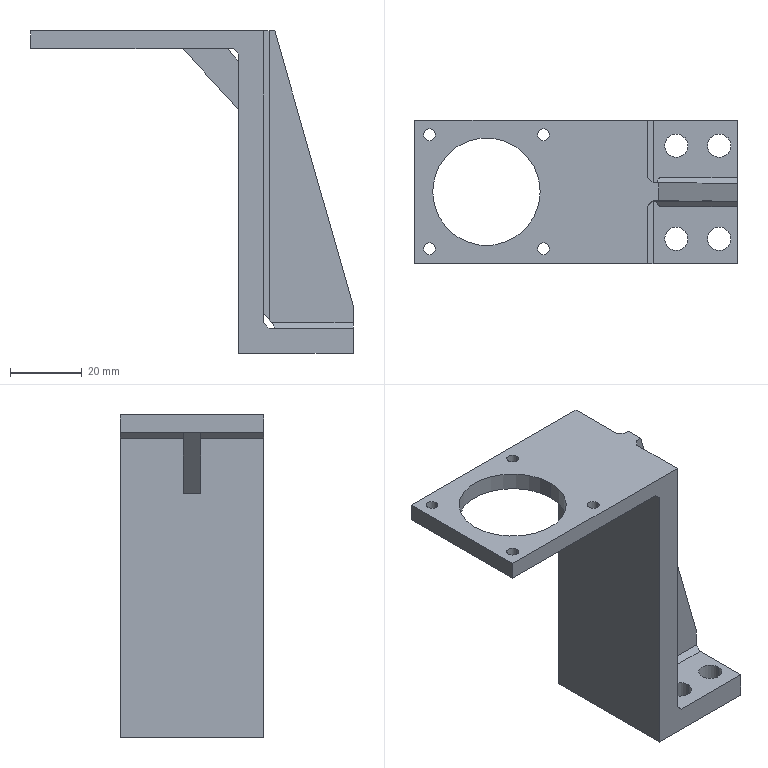Part | Creo | features CURVE 6, PROTRUSION 4, DATUM PLANE 3, CUT 2, CHAMFER 1, COORDINATE SYSTEM 1 | 1 solid | 42 faces | box 90 x 40 x 90 mm | volume 46256 mm3 | plane 24 | cylinder 18 | commonest cylinder face diameters 3.3 x8 6.5 x8 30 x2
STEP:
#1=CARTESIAN_POINT('',(0.,0.,0.));
#2=DIRECTION('',(0.,0.,1.));
#3=DIRECTION('',(1.,0.,0.));
#4=AXIS2_PLACEMENT_3D('',#1,#2,#3);
#5=CARTESIAN_POINT('',(36.5,-20.,0.));
#6=VERTEX_POINT('',#5);
#7=CARTESIAN_POINT('',(36.5,20.,0.));
#8=VERTEX_POINT('',#7);
#9=CARTESIAN_POINT('',(36.5,-20.,0.));
#10=DIRECTION('',(0.,1.,0.));
#11=VECTOR('',#10,40.);
#12=LINE('',#9,#11);
#13=EDGE_CURVE('',#6,#8,#12,.T.);
#14=ORIENTED_EDGE('',*,*,#13,.T.);
#15=CARTESIAN_POINT('',(-20.,20.,0.));
#16=VERTEX_POINT('',#15);
#17=CARTESIAN_POINT('',(36.5,20.,0.));
#18=DIRECTION('',(-1.,0.,0.));
#19=VECTOR('',#18,56.5);
#20=LINE('',#17,#19);
#21=EDGE_CURVE('',#8,#16,#20,.T.);
#22=ORIENTED_EDGE('',*,*,#21,.T.);
#23=CARTESIAN_POINT('',(-20.,-20.,0.));
#24=VERTEX_POINT('',#23);
#25=CARTESIAN_POINT('',(-20.,20.,0.));
#26=DIRECTION('',(0.,-1.,0.));
#27=VECTOR('',#26,40.);
#28=LINE('',#25,#27);
#29=EDGE_CURVE('',#16,#24,#28,.T.);
#30=ORIENTED_EDGE('',*,*,#29,.T.);
#31=CARTESIAN_POINT('',(-20.,-20.,0.));
#32=DIRECTION('',(1.,0.,0.));
#33=VECTOR('',#32,56.5);
#34=LINE('',#31,#33);
#35=EDGE_CURVE('',#24,#6,#34,.T.);
#36=ORIENTED_EDGE('',*,*,#35,.T.);
#37=EDGE_LOOP('',(#14,#22,#30,#36));
#38=FACE_OUTER_BOUND('',#37,.F.);
#39=CARTESIAN_POINT('',(17.56,15.91,0.));
#40=VERTEX_POINT('',#39);
#41=CARTESIAN_POINT('',(14.26,15.91,0.));
#42=VERTEX_POINT('',#41);
#43=CARTESIAN_POINT('',(15.91,15.91,0.));
#44=DIRECTION('',(0.,0.,-1.));
#45=DIRECTION('',(1.,0.,0.));
#46=AXIS2_PLACEMENT_3D('',#43,#44,#45);
#47=CIRCLE('',#46,1.65);
#48=EDGE_CURVE('',#40,#42,#47,.T.);
#49=ORIENTED_EDGE('',*,*,#48,.T.);
#50=CARTESIAN_POINT('',(15.91,15.91,0.));
#51=DIRECTION('',(0.,0.,-1.));
#52=DIRECTION('',(-1.,0.,0.));
#53=AXIS2_PLACEMENT_3D('',#50,#51,#52);
#54=CIRCLE('',#53,1.65);
#55=EDGE_CURVE('',#42,#40,#54,.T.);
#56=ORIENTED_EDGE('',*,*,#55,.T.);
#57=EDGE_LOOP('',(#49,#56));
#58=FACE_BOUND('',#57,.F.);
#59=CARTESIAN_POINT('',(-14.26,15.91,0.));
#60=VERTEX_POINT('',#59);
#61=CARTESIAN_POINT('',(-17.56,15.91,0.));
#62=VERTEX_POINT('',#61);
#63=CARTESIAN_POINT('',(-15.91,15.91,0.));
#64=DIRECTION('',(0.,0.,-1.));
#65=DIRECTION('',(1.,0.,0.));
#66=AXIS2_PLACEMENT_3D('',#63,#64,#65);
#67=CIRCLE('',#66,1.65);
#68=EDGE_CURVE('',#60,#62,#67,.T.);
#69=ORIENTED_EDGE('',*,*,#68,.T.);
#70=CARTESIAN_POINT('',(-15.91,15.91,0.));
#71=DIRECTION('',(0.,0.,-1.));
#72=DIRECTION('',(-1.,0.,0.));
#73=AXIS2_PLACEMENT_3D('',#70,#71,#72);
#74=CIRCLE('',#73,1.65);
#75=EDGE_CURVE('',#62,#60,#74,.T.);
#76=ORIENTED_EDGE('',*,*,#75,.T.);
#77=EDGE_LOOP('',(#69,#76));
#78=FACE_BOUND('',#77,.F.);
#79=CARTESIAN_POINT('',(-14.26,-15.91,0.));
#80=VERTEX_POINT('',#79);
#81=CARTESIAN_POINT('',(-17.56,-15.91,0.));
#82=VERTEX_POINT('',#81);
#83=CARTESIAN_POINT('',(-15.91,-15.91,0.));
#84=DIRECTION('',(0.,0.,-1.));
#85=DIRECTION('',(1.,0.,0.));
#86=AXIS2_PLACEMENT_3D('',#83,#84,#85);
#87=CIRCLE('',#86,1.65);
#88=EDGE_CURVE('',#80,#82,#87,.T.);
#89=ORIENTED_EDGE('',*,*,#88,.T.);
#90=CARTESIAN_POINT('',(-15.91,-15.91,0.));
#91=DIRECTION('',(0.,0.,-1.));
#92=DIRECTION('',(-1.,0.,0.));
#93=AXIS2_PLACEMENT_3D('',#90,#91,#92);
#94=CIRCLE('',#93,1.65);
#95=EDGE_CURVE('',#82,#80,#94,.T.);
#96=ORIENTED_EDGE('',*,*,#95,.T.);
#97=EDGE_LOOP('',(#89,#96));
#98=FACE_BOUND('',#97,.F.);
#99=CARTESIAN_POINT('',(17.56,-15.91,0.));
#100=VERTEX_POINT('',#99);
#101=CARTESIAN_POINT('',(14.26,-15.91,0.));
#102=VERTEX_POINT('',#101);
#103=CARTESIAN_POINT('',(15.91,-15.91,0.));
#104=DIRECTION('',(0.,0.,-1.));
#105=DIRECTION('',(1.,0.,0.));
#106=AXIS2_PLACEMENT_3D('',#103,#104,#105);
#107=CIRCLE('',#106,1.65);
#108=EDGE_CURVE('',#100,#102,#107,.T.);
#109=ORIENTED_EDGE('',*,*,#108,.T.);
#110=CARTESIAN_POINT('',(15.91,-15.91,0.));
#111=DIRECTION('',(0.,0.,-1.));
#112=DIRECTION('',(-1.,0.,0.));
#113=AXIS2_PLACEMENT_3D('',#110,#111,#112);
#114=CIRCLE('',#113,1.65);
#115=EDGE_CURVE('',#102,#100,#114,.T.);
#116=ORIENTED_EDGE('',*,*,#115,.T.);
#117=EDGE_LOOP('',(#109,#116));
#118=FACE_BOUND('',#117,.F.);
#119=CARTESIAN_POINT('',(34.828,-2.5,0.));
#120=VERTEX_POINT('',#119);
#121=CARTESIAN_POINT('',(22.404,-2.5,0.));
#122=VERTEX_POINT('',#121);
#123=CARTESIAN_POINT('',(34.828,-2.5,0.));
#124=DIRECTION('',(-1.,0.,0.));
#125=VECTOR('',#124,12.424);
#126=LINE('',#123,#125);
#127=EDGE_CURVE('',#120,#122,#126,.T.);
#128=ORIENTED_EDGE('',*,*,#127,.T.);
#129=CARTESIAN_POINT('',(22.404,2.5,0.));
#130=VERTEX_POINT('',#129);
#131=CARTESIAN_POINT('',(22.404,-2.5,0.));
#132=DIRECTION('',(0.,1.,0.));
#133=VECTOR('',#132,5.);
#134=LINE('',#131,#133);
#135=EDGE_CURVE('',#122,#130,#134,.T.);
#136=ORIENTED_EDGE('',*,*,#135,.T.);
#137=CARTESIAN_POINT('',(34.828,2.5,0.));
#138=VERTEX_POINT('',#137);
#139=CARTESIAN_POINT('',(34.828,2.5,0.));
#140=DIRECTION('',(-1.,0.,0.));
#141=VECTOR('',#140,12.424);
#142=LINE('',#139,#141);
#143=EDGE_CURVE('',#138,#130,#142,.T.);
#144=ORIENTED_EDGE('',*,*,#143,.F.);
#145=CARTESIAN_POINT('',(34.828,-2.5,0.));
#146=DIRECTION('',(0.,1.,0.));
#147=VECTOR('',#146,5.);
#148=LINE('',#145,#147);
#149=EDGE_CURVE('',#120,#138,#148,.T.);
#150=ORIENTED_EDGE('',*,*,#149,.F.);
#151=EDGE_LOOP('',(#128,#136,#144,#150));
#152=FACE_BOUND('',#151,.F.);
#153=CARTESIAN_POINT('',(15.,0.,0.));
#154=VERTEX_POINT('',#153);
#155=CARTESIAN_POINT('',(-15.,0.,0.));
#156=VERTEX_POINT('',#155);
#157=CARTESIAN_POINT('',(0.,0.,0.));
#158=DIRECTION('',(0.,0.,-1.));
#159=DIRECTION('',(1.,0.,0.));
#160=AXIS2_PLACEMENT_3D('',#157,#158,#159);
#161=CIRCLE('',#160,15.);
#162=EDGE_CURVE('',#154,#156,#161,.T.);
#163=ORIENTED_EDGE('',*,*,#162,.T.);
#164=CARTESIAN_POINT('',(0.,0.,0.));
#165=DIRECTION('',(0.,0.,-1.));
#166=DIRECTION('',(-1.,0.,0.));
#167=AXIS2_PLACEMENT_3D('',#164,#165,#166);
#168=CIRCLE('',#167,15.);
#169=EDGE_CURVE('',#156,#154,#168,.T.);
#170=ORIENTED_EDGE('',*,*,#169,.T.);
#171=EDGE_LOOP('',(#163,#170));
#172=FACE_BOUND('',#171,.F.);
#173=CARTESIAN_POINT('',(0.,0.,0.));
#174=DIRECTION('',(0.,0.,1.));
#175=DIRECTION('',(1.,0.,0.));
#176=AXIS2_PLACEMENT_3D('',#173,#174,#175);
#177=PLANE('',#176);
#178=ADVANCED_FACE('',(#38,#58,#78,#98,#118,#152,#172),#177,.F.);
#179=ORIENTED_EDGE('',*,*,#162,.F.);
#180=CARTESIAN_POINT('',(15.,0.,5.));
#181=VERTEX_POINT('',#180);
#182=CARTESIAN_POINT('',(15.,0.,0.));
#183=DIRECTION('',(0.,0.,1.));
#184=VECTOR('',#183,5.);
#185=LINE('',#182,#184);
#186=EDGE_CURVE('',#154,#181,#185,.T.);
#187=ORIENTED_EDGE('',*,*,#186,.T.);
#188=CARTESIAN_POINT('',(-15.,0.,5.));
#189=VERTEX_POINT('',#188);
#190=CARTESIAN_POINT('',(0.,0.,5.));
#191=DIRECTION('',(0.,0.,-1.));
#192=DIRECTION('',(1.,0.,0.));
#193=AXIS2_PLACEMENT_3D('',#190,#191,#192);
#194=CIRCLE('',#193,15.);
#195=EDGE_CURVE('',#181,#189,#194,.T.);
#196=ORIENTED_EDGE('',*,*,#195,.T.);
#197=CARTESIAN_POINT('',(-15.,0.,0.));
#198=DIRECTION('',(0.,0.,1.));
#199=VECTOR('',#198,5.);
#200=LINE('',#197,#199);
#201=EDGE_CURVE('',#156,#189,#200,.T.);
#202=ORIENTED_EDGE('',*,*,#201,.F.);
#203=EDGE_LOOP('',(#179,#187,#196,#202));
#204=FACE_OUTER_BOUND('',#203,.F.);
#205=CARTESIAN_POINT('',(0.,0.,0.));
#206=DIRECTION('',(0.,0.,1.));
#207=DIRECTION('',(1.,0.,0.));
#208=AXIS2_PLACEMENT_3D('',#205,#206,#207);
#209=CYLINDRICAL_SURFACE('',#208,15.);
#210=ADVANCED_FACE('',(#204),#209,.F.);
#211=ORIENTED_EDGE('',*,*,#169,.F.);
#212=ORIENTED_EDGE('',*,*,#201,.T.);
#213=CARTESIAN_POINT('',(0.,0.,5.));
#214=DIRECTION('',(0.,0.,-1.));
#215=DIRECTION('',(-1.,0.,0.));
#216=AXIS2_PLACEMENT_3D('',#213,#214,#215);
#217=CIRCLE('',#216,15.);
#218=EDGE_CURVE('',#189,#181,#217,.T.);
#219=ORIENTED_EDGE('',*,*,#218,.T.);
#220=ORIENTED_EDGE('',*,*,#186,.F.);
#221=EDGE_LOOP('',(#211,#212,#219,#220));
#222=FACE_OUTER_BOUND('',#221,.F.);
#223=CARTESIAN_POINT('',(0.,0.,0.));
#224=DIRECTION('',(0.,0.,1.));
#225=DIRECTION('',(1.,0.,0.));
#226=AXIS2_PLACEMENT_3D('',#223,#224,#225);
#227=CYLINDRICAL_SURFACE('',#226,15.);
#228=ADVANCED_FACE('',(#222),#227,.F.);
#229=CARTESIAN_POINT('',(45.,20.,5.));
#230=VERTEX_POINT('',#229);
#231=CARTESIAN_POINT('',(45.,4.,5.));
#232=VERTEX_POINT('',#231);
#233=CARTESIAN_POINT('',(45.,20.,5.));
#234=DIRECTION('',(0.,-1.,0.));
#235=VECTOR('',#234,16.);
#236=LINE('',#233,#235);
#237=EDGE_CURVE('',#230,#232,#236,.T.);
#238=ORIENTED_EDGE('',*,*,#237,.T.);
#239=CARTESIAN_POINT('',(46.5,2.5,5.));
#240=VERTEX_POINT('',#239);
#241=CARTESIAN_POINT('',(46.5,2.5,5.));
#242=DIRECTION('',(-0.7071,0.7071,0.));
#243=VECTOR('',#242,2.121);
#244=LINE('',#241,#243);
#245=EDGE_CURVE('',#240,#232,#244,.T.);
#246=ORIENTED_EDGE('',*,*,#245,.F.);
#247=CARTESIAN_POINT('',(48.097,2.5,5.));
#248=VERTEX_POINT('',#247);
#249=CARTESIAN_POINT('',(46.5,2.5,5.));
#250=DIRECTION('',(1.,0.,0.));
#251=VECTOR('',#250,1.597);
#252=LINE('',#249,#251);
#253=EDGE_CURVE('',#240,#248,#252,.T.);
#254=ORIENTED_EDGE('',*,*,#253,.T.);
#255=CARTESIAN_POINT('',(48.097,-2.5,5.));
#256=VERTEX_POINT('',#255);
#257=CARTESIAN_POINT('',(48.097,-2.5,5.));
#258=DIRECTION('',(0.,1.,0.));
#259=VECTOR('',#258,5.);
#260=LINE('',#257,#259);
#261=EDGE_CURVE('',#256,#248,#260,.T.);
#262=ORIENTED_EDGE('',*,*,#261,.F.);
#263=CARTESIAN_POINT('',(46.5,-2.5,5.));
#264=VERTEX_POINT('',#263);
#265=CARTESIAN_POINT('',(46.5,-2.5,5.));
#266=DIRECTION('',(1.,0.,0.));
#267=VECTOR('',#266,1.597);
#268=LINE('',#265,#267);
#269=EDGE_CURVE('',#264,#256,#268,.T.);
#270=ORIENTED_EDGE('',*,*,#269,.F.);
#271=CARTESIAN_POINT('',(45.,-4.,5.));
#272=VERTEX_POINT('',#271);
#273=CARTESIAN_POINT('',(45.,-4.,5.));
#274=DIRECTION('',(0.7071,0.7071,0.));
#275=VECTOR('',#274,2.121);
#276=LINE('',#273,#275);
#277=EDGE_CURVE('',#272,#264,#276,.T.);
#278=ORIENTED_EDGE('',*,*,#277,.F.);
#279=CARTESIAN_POINT('',(45.,-20.,5.));
#280=VERTEX_POINT('',#279);
#281=CARTESIAN_POINT('',(45.,-4.,5.));
#282=DIRECTION('',(0.,-1.,0.));
#283=VECTOR('',#282,16.);
#284=LINE('',#281,#283);
#285=EDGE_CURVE('',#272,#280,#284,.T.);
#286=ORIENTED_EDGE('',*,*,#285,.T.);
#287=CARTESIAN_POINT('',(-20.,-20.,5.));
#288=VERTEX_POINT('',#287);
#289=CARTESIAN_POINT('',(45.,-20.,5.));
#290=DIRECTION('',(-1.,0.,0.));
#291=VECTOR('',#290,65.);
#292=LINE('',#289,#291);
#293=EDGE_CURVE('',#280,#288,#292,.T.);
#294=ORIENTED_EDGE('',*,*,#293,.T.);
#295=CARTESIAN_POINT('',(-20.,20.,5.));
#296=VERTEX_POINT('',#295);
#297=CARTESIAN_POINT('',(-20.,20.,5.));
#298=DIRECTION('',(0.,-1.,0.));
#299=VECTOR('',#298,40.);
#300=LINE('',#297,#299);
#301=EDGE_CURVE('',#296,#288,#300,.T.);
#302=ORIENTED_EDGE('',*,*,#301,.F.);
#303=CARTESIAN_POINT('',(-20.,20.,5.));
#304=DIRECTION('',(1.,0.,0.));
#305=VECTOR('',#304,65.);
#306=LINE('',#303,#305);
#307=EDGE_CURVE('',#296,#230,#306,.T.);
#308=ORIENTED_EDGE('',*,*,#307,.T.);
#309=EDGE_LOOP('',(#238,#246,#254,#262,#270,#278,#286,#294,#302,#308));
#310=FACE_OUTER_BOUND('',#309,.F.);
#311=CARTESIAN_POINT('',(17.56,15.91,5.));
#312=VERTEX_POINT('',#311);
#313=CARTESIAN_POINT('',(14.26,15.91,5.));
#314=VERTEX_POINT('',#313);
#315=CARTESIAN_POINT('',(15.91,15.91,5.));
#316=DIRECTION('',(0.,0.,-1.));
#317=DIRECTION('',(1.,0.,0.));
#318=AXIS2_PLACEMENT_3D('',#315,#316,#317);
#319=CIRCLE('',#318,1.65);
#320=EDGE_CURVE('',#312,#314,#319,.T.);
#321=ORIENTED_EDGE('',*,*,#320,.F.);
#322=CARTESIAN_POINT('',(15.91,15.91,5.));
#323=DIRECTION('',(0.,0.,-1.));
#324=DIRECTION('',(-1.,0.,0.));
#325=AXIS2_PLACEMENT_3D('',#322,#323,#324);
#326=CIRCLE('',#325,1.65);
#327=EDGE_CURVE('',#314,#312,#326,.T.);
#328=ORIENTED_EDGE('',*,*,#327,.F.);
#329=EDGE_LOOP('',(#321,#328));
#330=FACE_BOUND('',#329,.F.);
#331=CARTESIAN_POINT('',(-14.26,15.91,5.));
#332=VERTEX_POINT('',#331);
#333=CARTESIAN_POINT('',(-17.56,15.91,5.));
#334=VERTEX_POINT('',#333);
#335=CARTESIAN_POINT('',(-15.91,15.91,5.));
#336=DIRECTION('',(0.,0.,-1.));
#337=DIRECTION('',(1.,0.,0.));
#338=AXIS2_PLACEMENT_3D('',#335,#336,#337);
#339=CIRCLE('',#338,1.65);
#340=EDGE_CURVE('',#332,#334,#339,.T.);
#341=ORIENTED_EDGE('',*,*,#340,.F.);
#342=CARTESIAN_POINT('',(-15.91,15.91,5.));
#343=DIRECTION('',(0.,0.,-1.));
#344=DIRECTION('',(-1.,0.,0.));
#345=AXIS2_PLACEMENT_3D('',#342,#343,#344);
#346=CIRCLE('',#345,1.65);
#347=EDGE_CURVE('',#334,#332,#346,.T.);
#348=ORIENTED_EDGE('',*,*,#347,.F.);
#349=EDGE_LOOP('',(#341,#348));
#350=FACE_BOUND('',#349,.F.);
#351=CARTESIAN_POINT('',(-14.26,-15.91,5.));
#352=VERTEX_POINT('',#351);
#353=CARTESIAN_POINT('',(-17.56,-15.91,5.));
#354=VERTEX_POINT('',#353);
#355=CARTESIAN_POINT('',(-15.91,-15.91,5.));
#356=DIRECTION('',(0.,0.,-1.));
#357=DIRECTION('',(1.,0.,0.));
#358=AXIS2_PLACEMENT_3D('',#355,#356,#357);
#359=CIRCLE('',#358,1.65);
#360=EDGE_CURVE('',#352,#354,#359,.T.);
#361=ORIENTED_EDGE('',*,*,#360,.F.);
#362=CARTESIAN_POINT('',(-15.91,-15.91,5.));
#363=DIRECTION('',(0.,0.,-1.));
#364=DIRECTION('',(-1.,0.,0.));
#365=AXIS2_PLACEMENT_3D('',#362,#363,#364);
#366=CIRCLE('',#365,1.65);
#367=EDGE_CURVE('',#354,#352,#366,.T.);
#368=ORIENTED_EDGE('',*,*,#367,.F.);
#369=EDGE_LOOP('',(#361,#368));
#370=FACE_BOUND('',#369,.F.);
#371=CARTESIAN_POINT('',(17.56,-15.91,5.));
#372=VERTEX_POINT('',#371);
#373=CARTESIAN_POINT('',(14.26,-15.91,5.));
#374=VERTEX_POINT('',#373);
#375=CARTESIAN_POINT('',(15.91,-15.91,5.));
#376=DIRECTION('',(0.,0.,-1.));
#377=DIRECTION('',(1.,0.,0.));
#378=AXIS2_PLACEMENT_3D('',#375,#376,#377);
#379=CIRCLE('',#378,1.65);
#380=EDGE_CURVE('',#372,#374,#379,.T.);
#381=ORIENTED_EDGE('',*,*,#380,.F.);
#382=CARTESIAN_POINT('',(15.91,-15.91,5.));
#383=DIRECTION('',(0.,0.,-1.));
#384=DIRECTION('',(-1.,0.,0.));
#385=AXIS2_PLACEMENT_3D('',#382,#383,#384);
#386=CIRCLE('',#385,1.65);
#387=EDGE_CURVE('',#374,#372,#386,.T.);
#388=ORIENTED_EDGE('',*,*,#387,.F.);
#389=EDGE_LOOP('',(#381,#388));
#390=FACE_BOUND('',#389,.F.);
#391=ORIENTED_EDGE('',*,*,#195,.F.);
#392=ORIENTED_EDGE('',*,*,#218,.F.);
#393=EDGE_LOOP('',(#391,#392));
#394=FACE_BOUND('',#393,.F.);
#395=CARTESIAN_POINT('',(0.,0.,5.));
#396=DIRECTION('',(0.,0.,1.));
#397=DIRECTION('',(1.,0.,0.));
#398=AXIS2_PLACEMENT_3D('',#395,#396,#397);
#399=PLANE('',#398);
#400=ADVANCED_FACE('',(#310,#330,#350,#370,#390,#394),#399,.T.);
#401=ORIENTED_EDGE('',*,*,#48,.F.);
#402=CARTESIAN_POINT('',(17.56,15.91,0.));
#403=DIRECTION('',(0.,0.,1.));
#404=VECTOR('',#403,5.);
#405=LINE('',#402,#404);
#406=EDGE_CURVE('',#40,#312,#405,.T.);
#407=ORIENTED_EDGE('',*,*,#406,.T.);
#408=ORIENTED_EDGE('',*,*,#320,.T.);
#409=CARTESIAN_POINT('',(14.26,15.91,0.));
#410=DIRECTION('',(0.,0.,1.));
#411=VECTOR('',#410,5.);
#412=LINE('',#409,#411);
#413=EDGE_CURVE('',#42,#314,#412,.T.);
#414=ORIENTED_EDGE('',*,*,#413,.F.);
#415=EDGE_LOOP('',(#401,#407,#408,#414));
#416=FACE_OUTER_BOUND('',#415,.F.);
#417=CARTESIAN_POINT('',(15.91,15.91,0.));
#418=DIRECTION('',(0.,0.,1.));
#419=DIRECTION('',(1.,0.,0.));
#420=AXIS2_PLACEMENT_3D('',#417,#418,#419);
#421=CYLINDRICAL_SURFACE('',#420,1.65);
#422=ADVANCED_FACE('',(#416),#421,.F.);
#423=ORIENTED_EDGE('',*,*,#55,.F.);
#424=ORIENTED_EDGE('',*,*,#413,.T.);
#425=ORIENTED_EDGE('',*,*,#327,.T.);
#426=ORIENTED_EDGE('',*,*,#406,.F.);
#427=EDGE_LOOP('',(#423,#424,#425,#426));
#428=FACE_OUTER_BOUND('',#427,.F.);
#429=CARTESIAN_POINT('',(15.91,15.91,0.));
#430=DIRECTION('',(0.,0.,1.));
#431=DIRECTION('',(1.,0.,0.));
#432=AXIS2_PLACEMENT_3D('',#429,#430,#431);
#433=CYLINDRICAL_SURFACE('',#432,1.65);
#434=ADVANCED_FACE('',(#428),#433,.F.);
#435=ORIENTED_EDGE('',*,*,#68,.F.);
#436=CARTESIAN_POINT('',(-14.26,15.91,0.));
#437=DIRECTION('',(0.,0.,1.));
#438=VECTOR('',#437,5.);
#439=LINE('',#436,#438);
#440=EDGE_CURVE('',#60,#332,#439,.T.);
#441=ORIENTED_EDGE('',*,*,#440,.T.);
#442=ORIENTED_EDGE('',*,*,#340,.T.);
#443=CARTESIAN_POINT('',(-17.56,15.91,0.));
#444=DIRECTION('',(0.,0.,1.));
#445=VECTOR('',#444,5.);
#446=LINE('',#443,#445);
#447=EDGE_CURVE('',#62,#334,#446,.T.);
#448=ORIENTED_EDGE('',*,*,#447,.F.);
#449=EDGE_LOOP('',(#435,#441,#442,#448));
#450=FACE_OUTER_BOUND('',#449,.F.);
#451=CARTESIAN_POINT('',(-15.91,15.91,0.));
#452=DIRECTION('',(0.,0.,1.));
#453=DIRECTION('',(1.,0.,0.));
#454=AXIS2_PLACEMENT_3D('',#451,#452,#453);
#455=CYLINDRICAL_SURFACE('',#454,1.65);
#456=ADVANCED_FACE('',(#450),#455,.F.);
#457=ORIENTED_EDGE('',*,*,#75,.F.);
#458=ORIENTED_EDGE('',*,*,#447,.T.);
#459=ORIENTED_EDGE('',*,*,#347,.T.);
#460=ORIENTED_EDGE('',*,*,#440,.F.);
#461=EDGE_LOOP('',(#457,#458,#459,#460));
#462=FACE_OUTER_BOUND('',#461,.F.);
#463=CARTESIAN_POINT('',(-15.91,15.91,0.));
#464=DIRECTION('',(0.,0.,1.));
#465=DIRECTION('',(1.,0.,0.));
#466=AXIS2_PLACEMENT_3D('',#463,#464,#465);
#467=CYLINDRICAL_SURFACE('',#466,1.65);
#468=ADVANCED_FACE('',(#462),#467,.F.);
#469=ORIENTED_EDGE('',*,*,#88,.F.);
#470=CARTESIAN_POINT('',(-14.26,-15.91,0.));
#471=DIRECTION('',(0.,0.,1.));
#472=VECTOR('',#471,5.);
#473=LINE('',#470,#472);
#474=EDGE_CURVE('',#80,#352,#473,.T.);
#475=ORIENTED_EDGE('',*,*,#474,.T.);
#476=ORIENTED_EDGE('',*,*,#360,.T.);
#477=CARTESIAN_POINT('',(-17.56,-15.91,0.));
#478=DIRECTION('',(0.,0.,1.));
#479=VECTOR('',#478,5.);
#480=LINE('',#477,#479);
#481=EDGE_CURVE('',#82,#354,#480,.T.);
#482=ORIENTED_EDGE('',*,*,#481,.F.);
#483=EDGE_LOOP('',(#469,#475,#476,#482));
#484=FACE_OUTER_BOUND('',#483,.F.);
#485=CARTESIAN_POINT('',(-15.91,-15.91,0.));
#486=DIRECTION('',(0.,0.,1.));
#487=DIRECTION('',(1.,0.,0.));
#488=AXIS2_PLACEMENT_3D('',#485,#486,#487);
#489=CYLINDRICAL_SURFACE('',#488,1.65);
#490=ADVANCED_FACE('',(#484),#489,.F.);
#491=ORIENTED_EDGE('',*,*,#95,.F.);
#492=ORIENTED_EDGE('',*,*,#481,.T.);
#493=ORIENTED_EDGE('',*,*,#367,.T.);
#494=ORIENTED_EDGE('',*,*,#474,.F.);
#495=EDGE_LOOP('',(#491,#492,#493,#494));
#496=FACE_OUTER_BOUND('',#495,.F.);
#497=CARTESIAN_POINT('',(-15.91,-15.91,0.));
#498=DIRECTION('',(0.,0.,1.));
#499=DIRECTION('',(1.,0.,0.));
#500=AXIS2_PLACEMENT_3D('',#497,#498,#499);
#501=CYLINDRICAL_SURFACE('',#500,1.65);
#502=ADVANCED_FACE('',(#496),#501,.F.);
#503=ORIENTED_EDGE('',*,*,#108,.F.);
#504=CARTESIAN_POINT('',(17.56,-15.91,0.));
#505=DIRECTION('',(0.,0.,1.));
#506=VECTOR('',#505,5.);
#507=LINE('',#504,#506);
#508=EDGE_CURVE('',#100,#372,#507,.T.);
#509=ORIENTED_EDGE('',*,*,#508,.T.);
#510=ORIENTED_EDGE('',*,*,#380,.T.);
#511=CARTESIAN_POINT('',(14.26,-15.91,0.));
#512=DIRECTION('',(0.,0.,1.));
#513=VECTOR('',#512,5.);
#514=LINE('',#511,#513);
#515=EDGE_CURVE('',#102,#374,#514,.T.);
#516=ORIENTED_EDGE('',*,*,#515,.F.);
#517=EDGE_LOOP('',(#503,#509,#510,#516));
#518=FACE_OUTER_BOUND('',#517,.F.);
#519=CARTESIAN_POINT('',(15.91,-15.91,0.));
#520=DIRECTION('',(0.,0.,1.));
#521=DIRECTION('',(1.,0.,0.));
#522=AXIS2_PLACEMENT_3D('',#519,#520,#521);
#523=CYLINDRICAL_SURFACE('',#522,1.65);
#524=ADVANCED_FACE('',(#518),#523,.F.);
#525=ORIENTED_EDGE('',*,*,#115,.F.);
#526=ORIENTED_EDGE('',*,*,#515,.T.);
#527=ORIENTED_EDGE('',*,*,#387,.T.);
#528=ORIENTED_EDGE('',*,*,#508,.F.);
#529=EDGE_LOOP('',(#525,#526,#527,#528));
#530=FACE_OUTER_BOUND('',#529,.F.);
#531=CARTESIAN_POINT('',(15.91,-15.91,0.));
#532=DIRECTION('',(0.,0.,1.));
#533=DIRECTION('',(1.,0.,0.));
#534=AXIS2_PLACEMENT_3D('',#531,#532,#533);
#535=CYLINDRICAL_SURFACE('',#534,1.65);
#536=ADVANCED_FACE('',(#530),#535,.F.);
#537=CARTESIAN_POINT('',(45.,20.,-76.5));
#538=VERTEX_POINT('',#537);
#539=CARTESIAN_POINT('',(45.,-20.,-76.5));
#540=VERTEX_POINT('',#539);
#541=CARTESIAN_POINT('',(45.,20.,-76.5));
#542=DIRECTION('',(0.,-1.,0.));
#543=VECTOR('',#542,40.);
#544=LINE('',#541,#543);
#545=EDGE_CURVE('',#538,#540,#544,.T.);
#546=ORIENTED_EDGE('',*,*,#545,.T.);
#547=CARTESIAN_POINT('',(45.,-20.,5.));
#548=DIRECTION('',(0.,0.,-1.));
#549=VECTOR('',#548,81.5);
#550=LINE('',#547,#549);
#551=EDGE_CURVE('',#280,#540,#550,.T.);
#552=ORIENTED_EDGE('',*,*,#551,.F.);
#553=ORIENTED_EDGE('',*,*,#285,.F.);
#554=CARTESIAN_POINT('',(45.,-4.,-73.824));
#555=VERTEX_POINT('',#554);
#556=CARTESIAN_POINT('',(45.,-4.,5.));
#557=DIRECTION('',(0.,0.,-1.));
#558=VECTOR('',#557,78.824);
#559=LINE('',#556,#558);
#560=EDGE_CURVE('',#272,#555,#559,.T.);
#561=ORIENTED_EDGE('',*,*,#560,.T.);
#562=CARTESIAN_POINT('',(45.,4.,-73.824));
#563=VERTEX_POINT('',#562);
#564=CARTESIAN_POINT('',(45.,4.,-73.824));
#565=DIRECTION('',(0.,-1.,0.));
#566=VECTOR('',#565,8.);
#567=LINE('',#564,#566);
#568=EDGE_CURVE('',#563,#555,#567,.T.);
#569=ORIENTED_EDGE('',*,*,#568,.F.);
#570=CARTESIAN_POINT('',(45.,4.,-73.824));
#571=DIRECTION('',(0.,0.,1.));
#572=VECTOR('',#571,78.824);
#573=LINE('',#570,#572);
#574=EDGE_CURVE('',#563,#232,#573,.T.);
#575=ORIENTED_EDGE('',*,*,#574,.T.);
#576=ORIENTED_EDGE('',*,*,#237,.F.);
#577=CARTESIAN_POINT('',(45.,20.,-76.5));
#578=DIRECTION('',(0.,0.,1.));
#579=VECTOR('',#578,81.5);
#580=LINE('',#577,#579);
#581=EDGE_CURVE('',#538,#230,#580,.T.);
#582=ORIENTED_EDGE('',*,*,#581,.F.);
#583=EDGE_LOOP('',(#546,#552,#553,#561,#569,#575,#576,#582));
#584=FACE_OUTER_BOUND('',#583,.F.);
#585=CARTESIAN_POINT('',(45.,0.,0.));
#586=DIRECTION('',(1.,0.,0.));
#587=DIRECTION('',(0.,1.,0.));
#588=AXIS2_PLACEMENT_3D('',#585,#586,#587);
#589=PLANE('',#588);
#590=ADVANCED_FACE('',(#584),#589,.T.);
#591=ORIENTED_EDGE('',*,*,#545,.F.);
#592=CARTESIAN_POINT('',(46.5,20.,-78.));
#593=VERTEX_POINT('',#592);
#594=CARTESIAN_POINT('',(45.,20.,-76.5));
#595=DIRECTION('',(0.7071,0.,-0.7071));
#596=VECTOR('',#595,2.121);
#597=LINE('',#594,#596);
#598=EDGE_CURVE('',#538,#593,#597,.T.);
#599=ORIENTED_EDGE('',*,*,#598,.T.);
#600=CARTESIAN_POINT('',(46.5,-20.,-78.));
#601=VERTEX_POINT('',#600);
#602=CARTESIAN_POINT('',(46.5,20.,-78.));
#603=DIRECTION('',(0.,-1.,0.));
#604=VECTOR('',#603,40.);
#605=LINE('',#602,#604);
#606=EDGE_CURVE('',#593,#601,#605,.T.);
#607=ORIENTED_EDGE('',*,*,#606,.T.);
#608=CARTESIAN_POINT('',(46.5,-20.,-78.));
#609=DIRECTION('',(-0.7071,0.,0.7071));
#610=VECTOR('',#609,2.121);
#611=LINE('',#608,#610);
#612=EDGE_CURVE('',#601,#540,#611,.T.);
#613=ORIENTED_EDGE('',*,*,#612,.T.);
#614=EDGE_LOOP('',(#591,#599,#607,#613));
#615=FACE_OUTER_BOUND('',#614,.F.);
#616=CARTESIAN_POINT('',(45.75,0.,-77.25));
#617=DIRECTION('',(0.7071,0.,0.7071));
#618=DIRECTION('',(-0.7071,0.,0.7071));
#619=AXIS2_PLACEMENT_3D('',#616,#617,#618);
#620=PLANE('',#619);
#621=ADVANCED_FACE('',(#615),#620,.T.);
#622=ORIENTED_EDGE('',*,*,#21,.F.);
#623=CARTESIAN_POINT('',(38.,20.,-1.5));
#624=VERTEX_POINT('',#623);
#625=CARTESIAN_POINT('',(38.,20.,-1.5));
#626=DIRECTION('',(-0.7071,0.,0.7071));
#627=VECTOR('',#626,2.121);
#628=LINE('',#625,#627);
#629=EDGE_CURVE('',#624,#8,#628,.T.);
#630=ORIENTED_EDGE('',*,*,#629,.F.);
#631=CARTESIAN_POINT('',(38.,20.,-85.));
#632=VERTEX_POINT('',#631);
#633=CARTESIAN_POINT('',(38.,20.,-85.));
#634=DIRECTION('',(0.,0.,1.));
#635=VECTOR('',#634,83.5);
#636=LINE('',#633,#635);
#637=EDGE_CURVE('',#632,#624,#636,.T.);
#638=ORIENTED_EDGE('',*,*,#637,.F.);
#639=CARTESIAN_POINT('',(70.,20.,-85.));
#640=VERTEX_POINT('',#639);
#641=CARTESIAN_POINT('',(38.,20.,-85.));
#642=DIRECTION('',(1.,0.,0.));
#643=VECTOR('',#642,32.);
#644=LINE('',#641,#643);
#645=EDGE_CURVE('',#632,#640,#644,.T.);
#646=ORIENTED_EDGE('',*,*,#645,.T.);
#647=CARTESIAN_POINT('',(70.,20.,-78.));
#648=VERTEX_POINT('',#647);
#649=CARTESIAN_POINT('',(70.,20.,-85.));
#650=DIRECTION('',(0.,0.,1.));
#651=VECTOR('',#650,7.);
#652=LINE('',#649,#651);
#653=EDGE_CURVE('',#640,#648,#652,.T.);
#654=ORIENTED_EDGE('',*,*,#653,.T.);
#655=CARTESIAN_POINT('',(46.5,20.,-78.));
#656=DIRECTION('',(1.,0.,0.));
#657=VECTOR('',#656,23.5);
#658=LINE('',#655,#657);
#659=EDGE_CURVE('',#593,#648,#658,.T.);
#660=ORIENTED_EDGE('',*,*,#659,.F.);
#661=ORIENTED_EDGE('',*,*,#598,.F.);
#662=ORIENTED_EDGE('',*,*,#581,.T.);
#663=ORIENTED_EDGE('',*,*,#307,.F.);
#664=CARTESIAN_POINT('',(-20.,20.,0.));
#665=DIRECTION('',(0.,0.,1.));
#666=VECTOR('',#665,5.);
#667=LINE('',#664,#666);
#668=EDGE_CURVE('',#16,#296,#667,.T.);
#669=ORIENTED_EDGE('',*,*,#668,.F.);
#670=EDGE_LOOP('',(#622,#630,#638,#646,#654,#660,#661,#662,#663,#669));
#671=FACE_OUTER_BOUND('',#670,.F.);
#672=CARTESIAN_POINT('',(20.,20.,0.));
#673=DIRECTION('',(0.,1.,0.));
#674=DIRECTION('',(-1.,0.,0.));
#675=AXIS2_PLACEMENT_3D('',#672,#673,#674);
#676=PLANE('',#675);
#677=ADVANCED_FACE('',(#671),#676,.T.);
#678=ORIENTED_EDGE('',*,*,#13,.F.);
#679=CARTESIAN_POINT('',(38.,-20.,-1.5));
#680=VERTEX_POINT('',#679);
#681=CARTESIAN_POINT('',(36.5,-20.,0.));
#682=DIRECTION('',(0.7071,0.,-0.7071));
#683=VECTOR('',#682,2.121);
#684=LINE('',#681,#683);
#685=EDGE_CURVE('',#6,#680,#684,.T.);
#686=ORIENTED_EDGE('',*,*,#685,.T.);
#687=CARTESIAN_POINT('',(38.,-20.,-1.5));
#688=DIRECTION('',(0.,1.,0.));
#689=VECTOR('',#688,40.);
#690=LINE('',#687,#689);
#691=EDGE_CURVE('',#680,#624,#690,.T.);
#692=ORIENTED_EDGE('',*,*,#691,.T.);
#693=ORIENTED_EDGE('',*,*,#629,.T.);
#694=EDGE_LOOP('',(#678,#686,#692,#693));
#695=FACE_OUTER_BOUND('',#694,.F.);
#696=CARTESIAN_POINT('',(37.25,0.,-0.75));
#697=DIRECTION('',(-0.7071,0.,-0.7071));
#698=DIRECTION('',(-0.7071,0.,0.7071));
#699=AXIS2_PLACEMENT_3D('',#696,#697,#698);
#700=PLANE('',#699);
#701=ADVANCED_FACE('',(#695),#700,.T.);
#702=CARTESIAN_POINT('',(38.,-20.,-85.));
#703=VERTEX_POINT('',#702);
#704=CARTESIAN_POINT('',(38.,-20.,-85.));
#705=DIRECTION('',(0.,0.,1.));
#706=VECTOR('',#705,83.5);
#707=LINE('',#704,#706);
#708=EDGE_CURVE('',#703,#680,#707,.T.);
#709=ORIENTED_EDGE('',*,*,#708,.T.);
#710=ORIENTED_EDGE('',*,*,#685,.F.);
#711=ORIENTED_EDGE('',*,*,#35,.F.);
#712=CARTESIAN_POINT('',(-20.,-20.,0.));
#713=DIRECTION('',(0.,0.,1.));
#714=VECTOR('',#713,5.);
#715=LINE('',#712,#714);
#716=EDGE_CURVE('',#24,#288,#715,.T.);
#717=ORIENTED_EDGE('',*,*,#716,.T.);
#718=ORIENTED_EDGE('',*,*,#293,.F.);
#719=ORIENTED_EDGE('',*,*,#551,.T.);
#720=ORIENTED_EDGE('',*,*,#612,.F.);
#721=CARTESIAN_POINT('',(70.,-20.,-78.));
#722=VERTEX_POINT('',#721);
#723=CARTESIAN_POINT('',(46.5,-20.,-78.));
#724=DIRECTION('',(1.,0.,0.));
#725=VECTOR('',#724,23.5);
#726=LINE('',#723,#725);
#727=EDGE_CURVE('',#601,#722,#726,.T.);
#728=ORIENTED_EDGE('',*,*,#727,.T.);
#729=CARTESIAN_POINT('',(70.,-20.,-85.));
#730=VERTEX_POINT('',#729);
#731=CARTESIAN_POINT('',(70.,-20.,-78.));
#732=DIRECTION('',(0.,0.,-1.));
#733=VECTOR('',#732,7.);
#734=LINE('',#731,#733);
#735=EDGE_CURVE('',#722,#730,#734,.T.);
#736=ORIENTED_EDGE('',*,*,#735,.T.);
#737=CARTESIAN_POINT('',(70.,-20.,-85.));
#738=DIRECTION('',(-1.,0.,0.));
#739=VECTOR('',#738,32.);
#740=LINE('',#737,#739);
#741=EDGE_CURVE('',#730,#703,#740,.T.);
#742=ORIENTED_EDGE('',*,*,#741,.T.);
#743=EDGE_LOOP('',(#709,#710,#711,#717,#718,#719,#720,#728,#736,#742));
#744=FACE_OUTER_BOUND('',#743,.F.);
#745=CARTESIAN_POINT('',(-20.,-20.,0.));
#746=DIRECTION('',(0.,-1.,0.));
#747=DIRECTION('',(1.,0.,0.));
#748=AXIS2_PLACEMENT_3D('',#745,#746,#747);
#749=PLANE('',#748);
#750=ADVANCED_FACE('',(#744),#749,.T.);
#751=ORIENTED_EDGE('',*,*,#691,.F.);
#752=ORIENTED_EDGE('',*,*,#708,.F.);
#753=CARTESIAN_POINT('',(38.,-20.,-85.));
#754=DIRECTION('',(0.,1.,0.));
#755=VECTOR('',#754,40.);
#756=LINE('',#753,#755);
#757=EDGE_CURVE('',#703,#632,#756,.T.);
#758=ORIENTED_EDGE('',*,*,#757,.T.);
#759=ORIENTED_EDGE('',*,*,#637,.T.);
#760=EDGE_LOOP('',(#751,#752,#758,#759));
#761=FACE_OUTER_BOUND('',#760,.F.);
#762=CARTESIAN_POINT('',(38.,-2.5,-3.453));
#763=VERTEX_POINT('',#762);
#764=CARTESIAN_POINT('',(38.,-2.5,-16.975));
#765=VERTEX_POINT('',#764);
#766=CARTESIAN_POINT('',(38.,-2.5,-3.453));
#767=DIRECTION('',(0.,0.,-1.));
#768=VECTOR('',#767,13.522);
#769=LINE('',#766,#768);
#770=EDGE_CURVE('',#763,#765,#769,.T.);
#771=ORIENTED_EDGE('',*,*,#770,.F.);
#772=CARTESIAN_POINT('',(38.,2.5,-3.453));
#773=VERTEX_POINT('',#772);
#774=CARTESIAN_POINT('',(38.,-2.5,-3.453));
#775=DIRECTION('',(0.,1.,0.));
#776=VECTOR('',#775,5.);
#777=LINE('',#774,#776);
#778=EDGE_CURVE('',#763,#773,#777,.T.);
#779=ORIENTED_EDGE('',*,*,#778,.T.);
#780=CARTESIAN_POINT('',(38.,2.5,-16.975));
#781=VERTEX_POINT('',#780);
#782=CARTESIAN_POINT('',(38.,2.5,-3.453));
#783=DIRECTION('',(0.,0.,-1.));
#784=VECTOR('',#783,13.522);
#785=LINE('',#782,#784);
#786=EDGE_CURVE('',#773,#781,#785,.T.);
#787=ORIENTED_EDGE('',*,*,#786,.T.);
#788=CARTESIAN_POINT('',(38.,-2.5,-16.975));
#789=DIRECTION('',(0.,1.,0.));
#790=VECTOR('',#789,5.);
#791=LINE('',#788,#790);
#792=EDGE_CURVE('',#765,#781,#791,.T.);
#793=ORIENTED_EDGE('',*,*,#792,.F.);
#794=EDGE_LOOP('',(#771,#779,#787,#793));
#795=FACE_BOUND('',#794,.F.);
#796=CARTESIAN_POINT('',(38.,-20.,-85.));
#797=DIRECTION('',(1.,0.,0.));
#798=DIRECTION('',(0.,0.,1.));
#799=AXIS2_PLACEMENT_3D('',#796,#797,#798);
#800=PLANE('',#799);
#801=ADVANCED_FACE('',(#761,#795),#800,.F.);
#802=ORIENTED_EDGE('',*,*,#127,.F.);
#803=CARTESIAN_POINT('',(34.828,-2.5,0.));
#804=DIRECTION('',(0.6766,0.,-0.7364));
#805=VECTOR('',#804,4.689);
#806=LINE('',#803,#805);
#807=EDGE_CURVE('',#120,#763,#806,.T.);
#808=ORIENTED_EDGE('',*,*,#807,.T.);
#809=ORIENTED_EDGE('',*,*,#770,.T.);
#810=CARTESIAN_POINT('',(38.,-2.5,-16.975));
#811=DIRECTION('',(-0.6766,0.,0.7364));
#812=VECTOR('',#811,23.052);
#813=LINE('',#810,#812);
#814=EDGE_CURVE('',#765,#122,#813,.T.);
#815=ORIENTED_EDGE('',*,*,#814,.T.);
#816=EDGE_LOOP('',(#802,#808,#809,#815));
#817=FACE_OUTER_BOUND('',#816,.F.);
#818=CARTESIAN_POINT('',(0.,-2.5,0.));
#819=DIRECTION('',(0.,1.,0.));
#820=DIRECTION('',(0.,0.,-1.));
#821=AXIS2_PLACEMENT_3D('',#818,#819,#820);
#822=PLANE('',#821);
#823=ADVANCED_FACE('',(#817),#822,.F.);
#824=CARTESIAN_POINT('',(47.132,-2.5,-76.5));
#825=VERTEX_POINT('',#824);
#826=CARTESIAN_POINT('',(70.,-2.5,-76.5));
#827=VERTEX_POINT('',#826);
#828=CARTESIAN_POINT('',(47.132,-2.5,-76.5));
#829=DIRECTION('',(1.,0.,0.));
#830=VECTOR('',#829,22.868);
#831=LINE('',#828,#830);
#832=EDGE_CURVE('',#825,#827,#831,.T.);
#833=ORIENTED_EDGE('',*,*,#832,.F.);
#834=CARTESIAN_POINT('',(46.5,-2.5,-75.707));
#835=VERTEX_POINT('',#834);
#836=CARTESIAN_POINT('',(47.132,-2.5,-76.5));
#837=DIRECTION('',(-0.6232,0.,0.7821));
#838=VECTOR('',#837,1.014);
#839=LINE('',#836,#838);
#840=EDGE_CURVE('',#825,#835,#839,.T.);
#841=ORIENTED_EDGE('',*,*,#840,.T.);
#842=CARTESIAN_POINT('',(46.5,-2.5,5.));
#843=DIRECTION('',(0.,0.,-1.));
#844=VECTOR('',#843,80.707);
#845=LINE('',#842,#844);
#846=EDGE_CURVE('',#264,#835,#845,.T.);
#847=ORIENTED_EDGE('',*,*,#846,.F.);
#848=ORIENTED_EDGE('',*,*,#269,.T.);
#849=CARTESIAN_POINT('',(70.,-2.5,-71.745));
#850=VERTEX_POINT('',#849);
#851=CARTESIAN_POINT('',(48.097,-2.5,5.));
#852=DIRECTION('',(0.2744,0.,-0.9616));
#853=VECTOR('',#852,79.81);
#854=LINE('',#851,#853);
#855=EDGE_CURVE('',#256,#850,#854,.T.);
#856=ORIENTED_EDGE('',*,*,#855,.T.);
#857=CARTESIAN_POINT('',(70.,-2.5,-71.745));
#858=DIRECTION('',(0.,0.,-1.));
#859=VECTOR('',#858,4.755);
#860=LINE('',#857,#859);
#861=EDGE_CURVE('',#850,#827,#860,.T.);
#862=ORIENTED_EDGE('',*,*,#861,.T.);
#863=EDGE_LOOP('',(#833,#841,#847,#848,#856,#862));
#864=FACE_OUTER_BOUND('',#863,.F.);
#865=CARTESIAN_POINT('',(0.,-2.5,0.));
#866=DIRECTION('',(0.,1.,0.));
#867=DIRECTION('',(0.,0.,-1.));
#868=AXIS2_PLACEMENT_3D('',#865,#866,#867);
#869=PLANE('',#868);
#870=ADVANCED_FACE('',(#864),#869,.F.);
#871=ORIENTED_EDGE('',*,*,#149,.T.);
#872=CARTESIAN_POINT('',(34.828,2.5,0.));
#873=DIRECTION('',(0.6766,0.,-0.7364));
#874=VECTOR('',#873,4.689);
#875=LINE('',#872,#874);
#876=EDGE_CURVE('',#138,#773,#875,.T.);
#877=ORIENTED_EDGE('',*,*,#876,.T.);
#878=ORIENTED_EDGE('',*,*,#778,.F.);
#879=ORIENTED_EDGE('',*,*,#807,.F.);
#880=EDGE_LOOP('',(#871,#877,#878,#879));
#881=FACE_OUTER_BOUND('',#880,.F.);
#882=CARTESIAN_POINT('',(34.828,-2.5,0.));
#883=DIRECTION('',(0.7364,0.,0.6766));
#884=DIRECTION('',(0.6766,0.,-0.7364));
#885=AXIS2_PLACEMENT_3D('',#882,#883,#884);
#886=PLANE('',#885);
#887=ADVANCED_FACE('',(#881),#886,.T.);
#888=ORIENTED_EDGE('',*,*,#143,.T.);
#889=CARTESIAN_POINT('',(38.,2.5,-16.975));
#890=DIRECTION('',(-0.6766,0.,0.7364));
#891=VECTOR('',#890,23.052);
#892=LINE('',#889,#891);
#893=EDGE_CURVE('',#781,#130,#892,.T.);
#894=ORIENTED_EDGE('',*,*,#893,.F.);
#895=ORIENTED_EDGE('',*,*,#786,.F.);
#896=ORIENTED_EDGE('',*,*,#876,.F.);
#897=EDGE_LOOP('',(#888,#894,#895,#896));
#898=FACE_OUTER_BOUND('',#897,.F.);
#899=CARTESIAN_POINT('',(0.,2.5,0.));
#900=DIRECTION('',(0.,1.,0.));
#901=DIRECTION('',(0.,0.,-1.));
#902=AXIS2_PLACEMENT_3D('',#899,#900,#901);
#903=PLANE('',#902);
#904=ADVANCED_FACE('',(#898),#903,.T.);
#905=CARTESIAN_POINT('',(70.,2.5,-76.5));
#906=VERTEX_POINT('',#905);
#907=CARTESIAN_POINT('',(47.132,2.5,-76.5));
#908=VERTEX_POINT('',#907);
#909=CARTESIAN_POINT('',(70.,2.5,-76.5));
#910=DIRECTION('',(-1.,0.,0.));
#911=VECTOR('',#910,22.868);
#912=LINE('',#909,#911);
#913=EDGE_CURVE('',#906,#908,#912,.T.);
#914=ORIENTED_EDGE('',*,*,#913,.F.);
#915=CARTESIAN_POINT('',(70.,2.5,-71.745));
#916=VERTEX_POINT('',#915);
#917=CARTESIAN_POINT('',(70.,2.5,-71.745));
#918=DIRECTION('',(0.,0.,-1.));
#919=VECTOR('',#918,4.755);
#920=LINE('',#917,#919);
#921=EDGE_CURVE('',#916,#906,#920,.T.);
#922=ORIENTED_EDGE('',*,*,#921,.F.);
#923=CARTESIAN_POINT('',(48.097,2.5,5.));
#924=DIRECTION('',(0.2744,0.,-0.9616));
#925=VECTOR('',#924,79.81);
#926=LINE('',#923,#925);
#927=EDGE_CURVE('',#248,#916,#926,.T.);
#928=ORIENTED_EDGE('',*,*,#927,.F.);
#929=ORIENTED_EDGE('',*,*,#253,.F.);
#930=CARTESIAN_POINT('',(46.5,2.5,-75.707));
#931=VERTEX_POINT('',#930);
#932=CARTESIAN_POINT('',(46.5,2.5,-75.707));
#933=DIRECTION('',(0.,0.,1.));
#934=VECTOR('',#933,80.707);
#935=LINE('',#932,#934);
#936=EDGE_CURVE('',#931,#240,#935,.T.);
#937=ORIENTED_EDGE('',*,*,#936,.F.);
#938=CARTESIAN_POINT('',(47.132,2.5,-76.5));
#939=DIRECTION('',(-0.6232,0.,0.7821));
#940=VECTOR('',#939,1.014);
#941=LINE('',#938,#940);
#942=EDGE_CURVE('',#908,#931,#941,.T.);
#943=ORIENTED_EDGE('',*,*,#942,.F.);
#944=EDGE_LOOP('',(#914,#922,#928,#929,#937,#943));
#945=FACE_OUTER_BOUND('',#944,.F.);
#946=CARTESIAN_POINT('',(0.,2.5,0.));
#947=DIRECTION('',(0.,1.,0.));
#948=DIRECTION('',(0.,0.,-1.));
#949=AXIS2_PLACEMENT_3D('',#946,#947,#948);
#950=PLANE('',#949);
#951=ADVANCED_FACE('',(#945),#950,.T.);
#952=ORIENTED_EDGE('',*,*,#135,.F.);
#953=ORIENTED_EDGE('',*,*,#814,.F.);
#954=ORIENTED_EDGE('',*,*,#792,.T.);
#955=ORIENTED_EDGE('',*,*,#893,.T.);
#956=EDGE_LOOP('',(#952,#953,#954,#955));
#957=FACE_OUTER_BOUND('',#956,.F.);
#958=CARTESIAN_POINT('',(38.,-2.5,-16.975));
#959=DIRECTION('',(-0.7364,0.,-0.6766));
#960=DIRECTION('',(-0.6766,0.,0.7364));
#961=AXIS2_PLACEMENT_3D('',#958,#959,#960);
#962=PLANE('',#961);
#963=ADVANCED_FACE('',(#957),#962,.T.);
#964=CARTESIAN_POINT('',(70.,4.,-78.));
#965=VERTEX_POINT('',#964);
#966=CARTESIAN_POINT('',(48.327,4.,-78.));
#967=VERTEX_POINT('',#966);
#968=CARTESIAN_POINT('',(70.,4.,-78.));
#969=DIRECTION('',(-1.,0.,0.));
#970=VECTOR('',#969,21.673);
#971=LINE('',#968,#970);
#972=EDGE_CURVE('',#965,#967,#971,.T.);
#973=ORIENTED_EDGE('',*,*,#972,.F.);
#974=CARTESIAN_POINT('',(70.,4.,-78.));
#975=DIRECTION('',(0.,-0.7071,0.7071));
#976=VECTOR('',#975,2.121);
#977=LINE('',#974,#976);
#978=EDGE_CURVE('',#965,#906,#977,.T.);
#979=ORIENTED_EDGE('',*,*,#978,.T.);
#980=ORIENTED_EDGE('',*,*,#913,.T.);
#981=CARTESIAN_POINT('',(47.132,2.5,-76.5));
#982=DIRECTION('',(0.4909,0.616,-0.616));
#983=VECTOR('',#982,2.435);
#984=LINE('',#981,#983);
#985=EDGE_CURVE('',#908,#967,#984,.T.);
#986=ORIENTED_EDGE('',*,*,#985,.T.);
#987=EDGE_LOOP('',(#973,#979,#980,#986));
#988=FACE_OUTER_BOUND('',#987,.F.);
#989=CARTESIAN_POINT('',(58.566,3.25,-77.25));
#990=DIRECTION('',(0.,0.7071,0.7071));
#991=DIRECTION('',(0.,0.7071,-0.7071));
#992=AXIS2_PLACEMENT_3D('',#989,#990,#991);
#993=PLANE('',#992);
#994=ADVANCED_FACE('',(#988),#993,.T.);
#995=ORIENTED_EDGE('',*,*,#606,.F.);
#996=ORIENTED_EDGE('',*,*,#659,.T.);
#997=CARTESIAN_POINT('',(70.,20.,-78.));
#998=DIRECTION('',(0.,-1.,0.));
#999=VECTOR('',#998,16.);
#1000=LINE('',#997,#999);
#1001=EDGE_CURVE('',#648,#965,#1000,.T.);
#1002=ORIENTED_EDGE('',*,*,#1001,.T.);
#1003=ORIENTED_EDGE('',*,*,#972,.T.);
#1004=CARTESIAN_POINT('',(48.327,-4.,-78.));
#1005=VERTEX_POINT('',#1004);
#1006=CARTESIAN_POINT('',(48.327,-4.,-78.));
#1007=DIRECTION('',(0.,1.,0.));
#1008=VECTOR('',#1007,8.);
#1009=LINE('',#1006,#1008);
#1010=EDGE_CURVE('',#1005,#967,#1009,.T.);
#1011=ORIENTED_EDGE('',*,*,#1010,.F.);
#1012=CARTESIAN_POINT('',(70.,-4.,-78.));
#1013=VERTEX_POINT('',#1012);
#1014=CARTESIAN_POINT('',(48.327,-4.,-78.));
#1015=DIRECTION('',(1.,0.,0.));
#1016=VECTOR('',#1015,21.673);
#1017=LINE('',#1014,#1016);
#1018=EDGE_CURVE('',#1005,#1013,#1017,.T.);
#1019=ORIENTED_EDGE('',*,*,#1018,.T.);
#1020=CARTESIAN_POINT('',(70.,-4.,-78.));
#1021=DIRECTION('',(0.,-1.,0.));
#1022=VECTOR('',#1021,16.);
#1023=LINE('',#1020,#1022);
#1024=EDGE_CURVE('',#1013,#722,#1023,.T.);
#1025=ORIENTED_EDGE('',*,*,#1024,.T.);
#1026=ORIENTED_EDGE('',*,*,#727,.F.);
#1027=EDGE_LOOP('',(#995,#996,#1002,#1003,#1011,#1019,#1025,#1026));
#1028=FACE_OUTER_BOUND('',#1027,.F.);
#1029=CARTESIAN_POINT('',(56.25,13.,-78.));
#1030=VERTEX_POINT('',#1029);
#1031=CARTESIAN_POINT('',(49.75,13.,-78.));
#1032=VERTEX_POINT('',#1031);
#1033=CARTESIAN_POINT('',(53.,13.,-78.));
#1034=DIRECTION('',(0.,0.,1.));
#1035=DIRECTION('',(1.,0.,0.));
#1036=AXIS2_PLACEMENT_3D('',#1033,#1034,#1035);
#1037=CIRCLE('',#1036,3.25);
#1038=EDGE_CURVE('',#1030,#1032,#1037,.T.);
#1039=ORIENTED_EDGE('',*,*,#1038,.T.);
#1040=CARTESIAN_POINT('',(53.,13.,-78.));
#1041=DIRECTION('',(0.,0.,1.));
#1042=DIRECTION('',(-1.,0.,0.));
#1043=AXIS2_PLACEMENT_3D('',#1040,#1041,#1042);
#1044=CIRCLE('',#1043,3.25);
#1045=EDGE_CURVE('',#1032,#1030,#1044,.T.);
#1046=ORIENTED_EDGE('',*,*,#1045,.T.);
#1047=EDGE_LOOP('',(#1039,#1046));
#1048=FACE_BOUND('',#1047,.F.);
#1049=CARTESIAN_POINT('',(68.25,-13.,-78.));
#1050=VERTEX_POINT('',#1049);
#1051=CARTESIAN_POINT('',(61.75,-13.,-78.));
#1052=VERTEX_POINT('',#1051);
#1053=CARTESIAN_POINT('',(65.,-13.,-78.));
#1054=DIRECTION('',(0.,0.,1.));
#1055=DIRECTION('',(1.,0.,0.));
#1056=AXIS2_PLACEMENT_3D('',#1053,#1054,#1055);
#1057=CIRCLE('',#1056,3.25);
#1058=EDGE_CURVE('',#1050,#1052,#1057,.T.);
#1059=ORIENTED_EDGE('',*,*,#1058,.T.);
#1060=CARTESIAN_POINT('',(65.,-13.,-78.));
#1061=DIRECTION('',(0.,0.,1.));
#1062=DIRECTION('',(-1.,0.,0.));
#1063=AXIS2_PLACEMENT_3D('',#1060,#1061,#1062);
#1064=CIRCLE('',#1063,3.25);
#1065=EDGE_CURVE('',#1052,#1050,#1064,.T.);
#1066=ORIENTED_EDGE('',*,*,#1065,.T.);
#1067=EDGE_LOOP('',(#1059,#1066));
#1068=FACE_BOUND('',#1067,.F.);
#1069=CARTESIAN_POINT('',(56.25,-13.,-78.));
#1070=VERTEX_POINT('',#1069);
#1071=CARTESIAN_POINT('',(49.75,-13.,-78.));
#1072=VERTEX_POINT('',#1071);
#1073=CARTESIAN_POINT('',(53.,-13.,-78.));
#1074=DIRECTION('',(0.,0.,1.));
#1075=DIRECTION('',(1.,0.,0.));
#1076=AXIS2_PLACEMENT_3D('',#1073,#1074,#1075);
#1077=CIRCLE('',#1076,3.25);
#1078=EDGE_CURVE('',#1070,#1072,#1077,.T.);
#1079=ORIENTED_EDGE('',*,*,#1078,.T.);
#1080=CARTESIAN_POINT('',(53.,-13.,-78.));
#1081=DIRECTION('',(0.,0.,1.));
#1082=DIRECTION('',(-1.,0.,0.));
#1083=AXIS2_PLACEMENT_3D('',#1080,#1081,#1082);
#1084=CIRCLE('',#1083,3.25);
#1085=EDGE_CURVE('',#1072,#1070,#1084,.T.);
#1086=ORIENTED_EDGE('',*,*,#1085,.T.);
#1087=EDGE_LOOP('',(#1079,#1086));
#1088=FACE_BOUND('',#1087,.F.);
#1089=CARTESIAN_POINT('',(68.25,13.,-78.));
#1090=VERTEX_POINT('',#1089);
#1091=CARTESIAN_POINT('',(61.75,13.,-78.));
#1092=VERTEX_POINT('',#1091);
#1093=CARTESIAN_POINT('',(65.,13.,-78.));
#1094=DIRECTION('',(0.,0.,1.));
#1095=DIRECTION('',(1.,0.,0.));
#1096=AXIS2_PLACEMENT_3D('',#1093,#1094,#1095);
#1097=CIRCLE('',#1096,3.25);
#1098=EDGE_CURVE('',#1090,#1092,#1097,.T.);
#1099=ORIENTED_EDGE('',*,*,#1098,.T.);
#1100=CARTESIAN_POINT('',(65.,13.,-78.));
#1101=DIRECTION('',(0.,0.,1.));
#1102=DIRECTION('',(-1.,0.,0.));
#1103=AXIS2_PLACEMENT_3D('',#1100,#1101,#1102);
#1104=CIRCLE('',#1103,3.25);
#1105=EDGE_CURVE('',#1092,#1090,#1104,.T.);
#1106=ORIENTED_EDGE('',*,*,#1105,.T.);
#1107=EDGE_LOOP('',(#1099,#1106));
#1108=FACE_BOUND('',#1107,.F.);
#1109=CARTESIAN_POINT('',(45.,20.,-78.));
#1110=DIRECTION('',(0.,0.,1.));
#1111=DIRECTION('',(0.,-1.,0.));
#1112=AXIS2_PLACEMENT_3D('',#1109,#1110,#1111);
#1113=PLANE('',#1112);
#1114=ADVANCED_FACE('',(#1028,#1048,#1068,#1088,#1108),#1113,.T.);
#1115=CARTESIAN_POINT('',(68.25,13.,-85.));
#1116=VERTEX_POINT('',#1115);
#1117=CARTESIAN_POINT('',(61.75,13.,-85.));
#1118=VERTEX_POINT('',#1117);
#1119=CARTESIAN_POINT('',(65.,13.,-85.));
#1120=DIRECTION('',(0.,0.,1.));
#1121=DIRECTION('',(1.,0.,0.));
#1122=AXIS2_PLACEMENT_3D('',#1119,#1120,#1121);
#1123=CIRCLE('',#1122,3.25);
#1124=EDGE_CURVE('',#1116,#1118,#1123,.T.);
#1125=ORIENTED_EDGE('',*,*,#1124,.T.);
#1126=CARTESIAN_POINT('',(61.75,13.,-78.));
#1127=DIRECTION('',(0.,0.,-1.));
#1128=VECTOR('',#1127,7.);
#1129=LINE('',#1126,#1128);
#1130=EDGE_CURVE('',#1092,#1118,#1129,.T.);
#1131=ORIENTED_EDGE('',*,*,#1130,.F.);
#1132=ORIENTED_EDGE('',*,*,#1098,.F.);
#1133=CARTESIAN_POINT('',(68.25,13.,-78.));
#1134=DIRECTION('',(0.,0.,-1.));
#1135=VECTOR('',#1134,7.);
#1136=LINE('',#1133,#1135);
#1137=EDGE_CURVE('',#1090,#1116,#1136,.T.);
#1138=ORIENTED_EDGE('',*,*,#1137,.T.);
#1139=EDGE_LOOP('',(#1125,#1131,#1132,#1138));
#1140=FACE_OUTER_BOUND('',#1139,.F.);
#1141=CARTESIAN_POINT('',(65.,13.,-78.));
#1142=DIRECTION('',(0.,0.,1.));
#1143=DIRECTION('',(1.,0.,0.));
#1144=AXIS2_PLACEMENT_3D('',#1141,#1142,#1143);
#1145=CYLINDRICAL_SURFACE('',#1144,3.25);
#1146=ADVANCED_FACE('',(#1140),#1145,.F.);
#1147=ORIENTED_EDGE('',*,*,#741,.F.);
#1148=CARTESIAN_POINT('',(70.,-20.,-85.));
#1149=DIRECTION('',(0.,1.,0.));
#1150=VECTOR('',#1149,40.);
#1151=LINE('',#1148,#1150);
#1152=EDGE_CURVE('',#730,#640,#1151,.T.);
#1153=ORIENTED_EDGE('',*,*,#1152,.T.);
#1154=ORIENTED_EDGE('',*,*,#645,.F.);
#1155=ORIENTED_EDGE('',*,*,#757,.F.);
#1156=EDGE_LOOP('',(#1147,#1153,#1154,#1155));
#1157=FACE_OUTER_BOUND('',#1156,.F.);
#1158=ORIENTED_EDGE('',*,*,#1124,.F.);
#1159=CARTESIAN_POINT('',(65.,13.,-85.));
#1160=DIRECTION('',(0.,0.,1.));
#1161=DIRECTION('',(-1.,0.,0.));
#1162=AXIS2_PLACEMENT_3D('',#1159,#1160,#1161);
#1163=CIRCLE('',#1162,3.25);
#1164=EDGE_CURVE('',#1118,#1116,#1163,.T.);
#1165=ORIENTED_EDGE('',*,*,#1164,.F.);
#1166=EDGE_LOOP('',(#1158,#1165));
#1167=FACE_BOUND('',#1166,.F.);
#1168=CARTESIAN_POINT('',(56.25,13.,-85.));
#1169=VERTEX_POINT('',#1168);
#1170=CARTESIAN_POINT('',(49.75,13.,-85.));
#1171=VERTEX_POINT('',#1170);
#1172=CARTESIAN_POINT('',(53.,13.,-85.));
#1173=DIRECTION('',(0.,0.,1.));
#1174=DIRECTION('',(1.,0.,0.));
#1175=AXIS2_PLACEMENT_3D('',#1172,#1173,#1174);
#1176=CIRCLE('',#1175,3.25);
#1177=EDGE_CURVE('',#1169,#1171,#1176,.T.);
#1178=ORIENTED_EDGE('',*,*,#1177,.F.);
#1179=CARTESIAN_POINT('',(53.,13.,-85.));
#1180=DIRECTION('',(0.,0.,1.));
#1181=DIRECTION('',(-1.,0.,0.));
#1182=AXIS2_PLACEMENT_3D('',#1179,#1180,#1181);
#1183=CIRCLE('',#1182,3.25);
#1184=EDGE_CURVE('',#1171,#1169,#1183,.T.);
#1185=ORIENTED_EDGE('',*,*,#1184,.F.);
#1186=EDGE_LOOP('',(#1178,#1185));
#1187=FACE_BOUND('',#1186,.F.);
#1188=CARTESIAN_POINT('',(68.25,-13.,-85.));
#1189=VERTEX_POINT('',#1188);
#1190=CARTESIAN_POINT('',(61.75,-13.,-85.));
#1191=VERTEX_POINT('',#1190);
#1192=CARTESIAN_POINT('',(65.,-13.,-85.));
#1193=DIRECTION('',(0.,0.,1.));
#1194=DIRECTION('',(1.,0.,0.));
#1195=AXIS2_PLACEMENT_3D('',#1192,#1193,#1194);
#1196=CIRCLE('',#1195,3.25);
#1197=EDGE_CURVE('',#1189,#1191,#1196,.T.);
#1198=ORIENTED_EDGE('',*,*,#1197,.F.);
#1199=CARTESIAN_POINT('',(65.,-13.,-85.));
#1200=DIRECTION('',(0.,0.,1.));
#1201=DIRECTION('',(-1.,0.,0.));
#1202=AXIS2_PLACEMENT_3D('',#1199,#1200,#1201);
#1203=CIRCLE('',#1202,3.25);
#1204=EDGE_CURVE('',#1191,#1189,#1203,.T.);
#1205=ORIENTED_EDGE('',*,*,#1204,.F.);
#1206=EDGE_LOOP('',(#1198,#1205));
#1207=FACE_BOUND('',#1206,.F.);
#1208=CARTESIAN_POINT('',(56.25,-13.,-85.));
#1209=VERTEX_POINT('',#1208);
#1210=CARTESIAN_POINT('',(49.75,-13.,-85.));
#1211=VERTEX_POINT('',#1210);
#1212=CARTESIAN_POINT('',(53.,-13.,-85.));
#1213=DIRECTION('',(0.,0.,1.));
#1214=DIRECTION('',(1.,0.,0.));
#1215=AXIS2_PLACEMENT_3D('',#1212,#1213,#1214);
#1216=CIRCLE('',#1215,3.25);
#1217=EDGE_CURVE('',#1209,#1211,#1216,.T.);
#1218=ORIENTED_EDGE('',*,*,#1217,.F.);
#1219=CARTESIAN_POINT('',(53.,-13.,-85.));
#1220=DIRECTION('',(0.,0.,1.));
#1221=DIRECTION('',(-1.,0.,0.));
#1222=AXIS2_PLACEMENT_3D('',#1219,#1220,#1221);
#1223=CIRCLE('',#1222,3.25);
#1224=EDGE_CURVE('',#1211,#1209,#1223,.T.);
#1225=ORIENTED_EDGE('',*,*,#1224,.F.);
#1226=EDGE_LOOP('',(#1218,#1225));
#1227=FACE_BOUND('',#1226,.F.);
#1228=CARTESIAN_POINT('',(20.,-20.,-85.));
#1229=DIRECTION('',(0.,0.,-1.));
#1230=DIRECTION('',(0.,1.,0.));
#1231=AXIS2_PLACEMENT_3D('',#1228,#1229,#1230);
#1232=PLANE('',#1231);
#1233=ADVANCED_FACE('',(#1157,#1167,#1187,#1207,#1227),#1232,.T.);
#1234=ORIENTED_EDGE('',*,*,#1024,.F.);
#1235=CARTESIAN_POINT('',(70.,-2.5,-76.5));
#1236=DIRECTION('',(0.,-0.7071,-0.7071));
#1237=VECTOR('',#1236,2.121);
#1238=LINE('',#1235,#1237);
#1239=EDGE_CURVE('',#827,#1013,#1238,.T.);
#1240=ORIENTED_EDGE('',*,*,#1239,.F.);
#1241=ORIENTED_EDGE('',*,*,#861,.F.);
#1242=CARTESIAN_POINT('',(70.,-2.5,-71.745));
#1243=DIRECTION('',(0.,1.,0.));
#1244=VECTOR('',#1243,5.);
#1245=LINE('',#1242,#1244);
#1246=EDGE_CURVE('',#850,#916,#1245,.T.);
#1247=ORIENTED_EDGE('',*,*,#1246,.T.);
#1248=ORIENTED_EDGE('',*,*,#921,.T.);
#1249=ORIENTED_EDGE('',*,*,#978,.F.);
#1250=ORIENTED_EDGE('',*,*,#1001,.F.);
#1251=ORIENTED_EDGE('',*,*,#653,.F.);
#1252=ORIENTED_EDGE('',*,*,#1152,.F.);
#1253=ORIENTED_EDGE('',*,*,#735,.F.);
#1254=EDGE_LOOP('',(#1234,#1240,#1241,#1247,#1248,#1249,#1250,#1251,#1252,#1253));
#1255=FACE_OUTER_BOUND('',#1254,.F.);
#1256=CARTESIAN_POINT('',(70.,0.,0.));
#1257=DIRECTION('',(1.,0.,0.));
#1258=DIRECTION('',(0.,1.,0.));
#1259=AXIS2_PLACEMENT_3D('',#1256,#1257,#1258);
#1260=PLANE('',#1259);
#1261=ADVANCED_FACE('',(#1255),#1260,.T.);
#1262=ORIENTED_EDGE('',*,*,#1018,.F.);
#1263=CARTESIAN_POINT('',(48.327,-4.,-78.));
#1264=DIRECTION('',(-0.4909,0.616,0.616));
#1265=VECTOR('',#1264,2.435);
#1266=LINE('',#1263,#1265);
#1267=EDGE_CURVE('',#1005,#825,#1266,.T.);
#1268=ORIENTED_EDGE('',*,*,#1267,.T.);
#1269=ORIENTED_EDGE('',*,*,#832,.T.);
#1270=ORIENTED_EDGE('',*,*,#1239,.T.);
#1271=EDGE_LOOP('',(#1262,#1268,#1269,#1270));
#1272=FACE_OUTER_BOUND('',#1271,.F.);
#1273=CARTESIAN_POINT('',(58.566,-3.25,-77.25));
#1274=DIRECTION('',(0.,-0.7071,0.7071));
#1275=DIRECTION('',(0.,-0.7071,-0.7071));
#1276=AXIS2_PLACEMENT_3D('',#1273,#1274,#1275);
#1277=PLANE('',#1276);
#1278=ADVANCED_FACE('',(#1272),#1277,.T.);
#1279=ORIENTED_EDGE('',*,*,#840,.F.);
#1280=ORIENTED_EDGE('',*,*,#1267,.F.);
#1281=ORIENTED_EDGE('',*,*,#1010,.T.);
#1282=ORIENTED_EDGE('',*,*,#985,.F.);
#1283=ORIENTED_EDGE('',*,*,#942,.T.);
#1284=CARTESIAN_POINT('',(45.,4.,-73.824));
#1285=DIRECTION('',(0.5289,-0.5289,-0.6637));
#1286=VECTOR('',#1285,2.836);
#1287=LINE('',#1284,#1286);
#1288=EDGE_CURVE('',#563,#931,#1287,.T.);
#1289=ORIENTED_EDGE('',*,*,#1288,.F.);
#1290=ORIENTED_EDGE('',*,*,#568,.T.);
#1291=CARTESIAN_POINT('',(46.5,-2.5,-75.707));
#1292=DIRECTION('',(-0.5289,-0.5289,0.6637));
#1293=VECTOR('',#1292,2.836);
#1294=LINE('',#1291,#1293);
#1295=EDGE_CURVE('',#835,#555,#1294,.T.);
#1296=ORIENTED_EDGE('',*,*,#1295,.F.);
#1297=EDGE_LOOP('',(#1279,#1280,#1281,#1282,#1283,#1289,#1290,#1296));
#1298=FACE_OUTER_BOUND('',#1297,.F.);
#1299=CARTESIAN_POINT('',(48.327,-2.5,-78.));
#1300=DIRECTION('',(-0.7821,0.,-0.6232));
#1301=DIRECTION('',(-0.6232,0.,0.7821));
#1302=AXIS2_PLACEMENT_3D('',#1299,#1300,#1301);
#1303=PLANE('',#1302);
#1304=ADVANCED_FACE('',(#1298),#1303,.T.);
#1305=ORIENTED_EDGE('',*,*,#574,.F.);
#1306=ORIENTED_EDGE('',*,*,#1288,.T.);
#1307=ORIENTED_EDGE('',*,*,#936,.T.);
#1308=ORIENTED_EDGE('',*,*,#245,.T.);
#1309=EDGE_LOOP('',(#1305,#1306,#1307,#1308));
#1310=FACE_OUTER_BOUND('',#1309,.F.);
#1311=CARTESIAN_POINT('',(45.75,3.25,-35.353));
#1312=DIRECTION('',(0.7071,0.7071,0.));
#1313=DIRECTION('',(-0.7071,0.7071,0.));
#1314=AXIS2_PLACEMENT_3D('',#1311,#1312,#1313);
#1315=PLANE('',#1314);
#1316=ADVANCED_FACE('',(#1310),#1315,.T.);
#1317=ORIENTED_EDGE('',*,*,#560,.F.);
#1318=ORIENTED_EDGE('',*,*,#277,.T.);
#1319=ORIENTED_EDGE('',*,*,#846,.T.);
#1320=ORIENTED_EDGE('',*,*,#1295,.T.);
#1321=EDGE_LOOP('',(#1317,#1318,#1319,#1320));
#1322=FACE_OUTER_BOUND('',#1321,.F.);
#1323=CARTESIAN_POINT('',(45.75,-3.25,-35.353));
#1324=DIRECTION('',(0.7071,-0.7071,0.));
#1325=DIRECTION('',(-0.7071,-0.7071,0.));
#1326=AXIS2_PLACEMENT_3D('',#1323,#1324,#1325);
#1327=PLANE('',#1326);
#1328=ADVANCED_FACE('',(#1322),#1327,.T.);
#1329=ORIENTED_EDGE('',*,*,#855,.F.);
#1330=ORIENTED_EDGE('',*,*,#261,.T.);
#1331=ORIENTED_EDGE('',*,*,#927,.T.);
#1332=ORIENTED_EDGE('',*,*,#1246,.F.);
#1333=EDGE_LOOP('',(#1329,#1330,#1331,#1332));
#1334=FACE_OUTER_BOUND('',#1333,.F.);
#1335=CARTESIAN_POINT('',(48.097,-2.5,5.));
#1336=DIRECTION('',(0.9616,0.,0.2744));
#1337=DIRECTION('',(0.2744,0.,-0.9616));
#1338=AXIS2_PLACEMENT_3D('',#1335,#1336,#1337);
#1339=PLANE('',#1338);
#1340=ADVANCED_FACE('',(#1334),#1339,.T.);
#1341=ORIENTED_EDGE('',*,*,#1164,.T.);
#1342=ORIENTED_EDGE('',*,*,#1137,.F.);
#1343=ORIENTED_EDGE('',*,*,#1105,.F.);
#1344=ORIENTED_EDGE('',*,*,#1130,.T.);
#1345=EDGE_LOOP('',(#1341,#1342,#1343,#1344));
#1346=FACE_OUTER_BOUND('',#1345,.F.);
#1347=CARTESIAN_POINT('',(65.,13.,-78.));
#1348=DIRECTION('',(0.,0.,1.));
#1349=DIRECTION('',(1.,0.,0.));
#1350=AXIS2_PLACEMENT_3D('',#1347,#1348,#1349);
#1351=CYLINDRICAL_SURFACE('',#1350,3.25);
#1352=ADVANCED_FACE('',(#1346),#1351,.F.);
#1353=ORIENTED_EDGE('',*,*,#1177,.T.);
#1354=CARTESIAN_POINT('',(49.75,13.,-78.));
#1355=DIRECTION('',(0.,0.,-1.));
#1356=VECTOR('',#1355,7.);
#1357=LINE('',#1354,#1356);
#1358=EDGE_CURVE('',#1032,#1171,#1357,.T.);
#1359=ORIENTED_EDGE('',*,*,#1358,.F.);
#1360=ORIENTED_EDGE('',*,*,#1038,.F.);
#1361=CARTESIAN_POINT('',(56.25,13.,-78.));
#1362=DIRECTION('',(0.,0.,-1.));
#1363=VECTOR('',#1362,7.);
#1364=LINE('',#1361,#1363);
#1365=EDGE_CURVE('',#1030,#1169,#1364,.T.);
#1366=ORIENTED_EDGE('',*,*,#1365,.T.);
#1367=EDGE_LOOP('',(#1353,#1359,#1360,#1366));
#1368=FACE_OUTER_BOUND('',#1367,.F.);
#1369=CARTESIAN_POINT('',(53.,13.,-78.));
#1370=DIRECTION('',(0.,0.,1.));
#1371=DIRECTION('',(1.,0.,0.));
#1372=AXIS2_PLACEMENT_3D('',#1369,#1370,#1371);
#1373=CYLINDRICAL_SURFACE('',#1372,3.25);
#1374=ADVANCED_FACE('',(#1368),#1373,.F.);
#1375=ORIENTED_EDGE('',*,*,#1184,.T.);
#1376=ORIENTED_EDGE('',*,*,#1365,.F.);
#1377=ORIENTED_EDGE('',*,*,#1045,.F.);
#1378=ORIENTED_EDGE('',*,*,#1358,.T.);
#1379=EDGE_LOOP('',(#1375,#1376,#1377,#1378));
#1380=FACE_OUTER_BOUND('',#1379,.F.);
#1381=CARTESIAN_POINT('',(53.,13.,-78.));
#1382=DIRECTION('',(0.,0.,1.));
#1383=DIRECTION('',(1.,0.,0.));
#1384=AXIS2_PLACEMENT_3D('',#1381,#1382,#1383);
#1385=CYLINDRICAL_SURFACE('',#1384,3.25);
#1386=ADVANCED_FACE('',(#1380),#1385,.F.);
#1387=ORIENTED_EDGE('',*,*,#1197,.T.);
#1388=CARTESIAN_POINT('',(61.75,-13.,-78.));
#1389=DIRECTION('',(0.,0.,-1.));
#1390=VECTOR('',#1389,7.);
#1391=LINE('',#1388,#1390);
#1392=EDGE_CURVE('',#1052,#1191,#1391,.T.);
#1393=ORIENTED_EDGE('',*,*,#1392,.F.);
#1394=ORIENTED_EDGE('',*,*,#1058,.F.);
#1395=CARTESIAN_POINT('',(68.25,-13.,-78.));
#1396=DIRECTION('',(0.,0.,-1.));
#1397=VECTOR('',#1396,7.);
#1398=LINE('',#1395,#1397);
#1399=EDGE_CURVE('',#1050,#1189,#1398,.T.);
#1400=ORIENTED_EDGE('',*,*,#1399,.T.);
#1401=EDGE_LOOP('',(#1387,#1393,#1394,#1400));
#1402=FACE_OUTER_BOUND('',#1401,.F.);
#1403=CARTESIAN_POINT('',(65.,-13.,-78.));
#1404=DIRECTION('',(0.,0.,1.));
#1405=DIRECTION('',(1.,0.,0.));
#1406=AXIS2_PLACEMENT_3D('',#1403,#1404,#1405);
#1407=CYLINDRICAL_SURFACE('',#1406,3.25);
#1408=ADVANCED_FACE('',(#1402),#1407,.F.);
#1409=ORIENTED_EDGE('',*,*,#1204,.T.);
#1410=ORIENTED_EDGE('',*,*,#1399,.F.);
#1411=ORIENTED_EDGE('',*,*,#1065,.F.);
#1412=ORIENTED_EDGE('',*,*,#1392,.T.);
#1413=EDGE_LOOP('',(#1409,#1410,#1411,#1412));
#1414=FACE_OUTER_BOUND('',#1413,.F.);
#1415=CARTESIAN_POINT('',(65.,-13.,-78.));
#1416=DIRECTION('',(0.,0.,1.));
#1417=DIRECTION('',(1.,0.,0.));
#1418=AXIS2_PLACEMENT_3D('',#1415,#1416,#1417);
#1419=CYLINDRICAL_SURFACE('',#1418,3.25);
#1420=ADVANCED_FACE('',(#1414),#1419,.F.);
#1421=ORIENTED_EDGE('',*,*,#1217,.T.);
#1422=CARTESIAN_POINT('',(49.75,-13.,-78.));
#1423=DIRECTION('',(0.,0.,-1.));
#1424=VECTOR('',#1423,7.);
#1425=LINE('',#1422,#1424);
#1426=EDGE_CURVE('',#1072,#1211,#1425,.T.);
#1427=ORIENTED_EDGE('',*,*,#1426,.F.);
#1428=ORIENTED_EDGE('',*,*,#1078,.F.);
#1429=CARTESIAN_POINT('',(56.25,-13.,-78.));
#1430=DIRECTION('',(0.,0.,-1.));
#1431=VECTOR('',#1430,7.);
#1432=LINE('',#1429,#1431);
#1433=EDGE_CURVE('',#1070,#1209,#1432,.T.);
#1434=ORIENTED_EDGE('',*,*,#1433,.T.);
#1435=EDGE_LOOP('',(#1421,#1427,#1428,#1434));
#1436=FACE_OUTER_BOUND('',#1435,.F.);
#1437=CARTESIAN_POINT('',(53.,-13.,-78.));
#1438=DIRECTION('',(0.,0.,1.));
#1439=DIRECTION('',(1.,0.,0.));
#1440=AXIS2_PLACEMENT_3D('',#1437,#1438,#1439);
#1441=CYLINDRICAL_SURFACE('',#1440,3.25);
#1442=ADVANCED_FACE('',(#1436),#1441,.F.);
#1443=ORIENTED_EDGE('',*,*,#1224,.T.);
#1444=ORIENTED_EDGE('',*,*,#1433,.F.);
#1445=ORIENTED_EDGE('',*,*,#1085,.F.);
#1446=ORIENTED_EDGE('',*,*,#1426,.T.);
#1447=EDGE_LOOP('',(#1443,#1444,#1445,#1446));
#1448=FACE_OUTER_BOUND('',#1447,.F.);
#1449=CARTESIAN_POINT('',(53.,-13.,-78.));
#1450=DIRECTION('',(0.,0.,1.));
#1451=DIRECTION('',(1.,0.,0.));
#1452=AXIS2_PLACEMENT_3D('',#1449,#1450,#1451);
#1453=CYLINDRICAL_SURFACE('',#1452,3.25);
#1454=ADVANCED_FACE('',(#1448),#1453,.F.);
#1455=ORIENTED_EDGE('',*,*,#29,.F.);
#1456=ORIENTED_EDGE('',*,*,#668,.T.);
#1457=ORIENTED_EDGE('',*,*,#301,.T.);
#1458=ORIENTED_EDGE('',*,*,#716,.F.);
#1459=EDGE_LOOP('',(#1455,#1456,#1457,#1458));
#1460=FACE_OUTER_BOUND('',#1459,.F.);
#1461=CARTESIAN_POINT('',(-20.,20.,0.));
#1462=DIRECTION('',(-1.,0.,0.));
#1463=DIRECTION('',(0.,-1.,0.));
#1464=AXIS2_PLACEMENT_3D('',#1461,#1462,#1463);
#1465=PLANE('',#1464);
#1466=ADVANCED_FACE('',(#1460),#1465,.T.);
#1467=CLOSED_SHELL('',(#178,#210,#228,#400,#422,#434,#456,#468,#490,#502,#524,#536,#590,#621,#677,#701,#750,#801,#823,#870,#887,#904,#951,#963,#994,#1114,#1146,#1233,#1261,#1278,#1304,#1316,#1328,#1340,#1352,#1374,#1386,#1408,#1420,#1442,#1454,#1466));
#1468=MANIFOLD_SOLID_BREP('',#1467);
#1469=(LENGTH_UNIT()NAMED_UNIT(*)SI_UNIT(.MILLI.,.METRE.));
#1470=UNCERTAINTY_MEASURE_WITH_UNIT(LENGTH_MEASURE(0.01334),#1469,'','');
#1471=(NAMED_UNIT(*)PLANE_ANGLE_UNIT()SI_UNIT($,.RADIAN.));
#1472=PLANE_ANGLE_MEASURE_WITH_UNIT(PLANE_ANGLE_MEASURE(0.01745),#1471);
#1473=(CONVERSION_BASED_UNIT('DEGREE',#1472)NAMED_UNIT(*)PLANE_ANGLE_UNIT());
#1474=(NAMED_UNIT(*)SI_UNIT($,.STERADIAN.)SOLID_ANGLE_UNIT());
#1475=(GEOMETRIC_REPRESENTATION_CONTEXT(3)GLOBAL_UNCERTAINTY_ASSIGNED_CONTEXT((#1470))GLOBAL_UNIT_ASSIGNED_CONTEXT((#1469,#1473,#1474))REPRESENTATION_CONTEXT('',''));
#1476=ADVANCED_BREP_SHAPE_REPRESENTATION('',(#4,#1468),#1475);